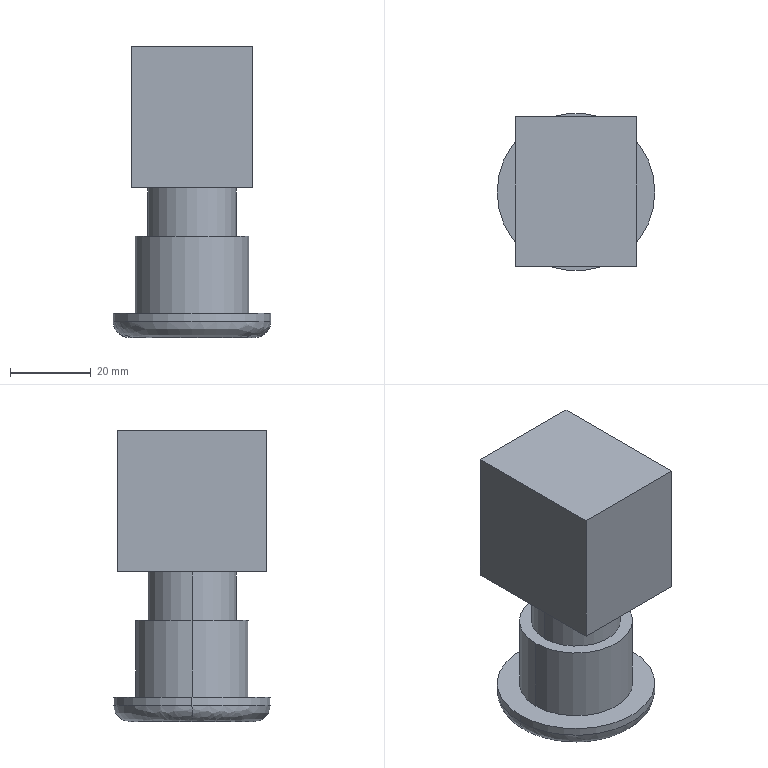Part | STEP file | Stop button AS2201 | 1 solid | 17 faces | box 39 x 39 x 72 mm | volume 61878 mm3 | plane 9 | cylinder 6 | spline 2 | commonest cylinder face diameters 22 x2 28 x2 39 x2
STEP:
#1=CARTESIAN_POINT('',(-15.5,0.,-6.));
#2=VERTEX_POINT('',#1);
#3=CARTESIAN_POINT('',(15.5,0.,-6.));
#4=VERTEX_POINT('',#3);
#5=CARTESIAN_POINT('',(-15.5,0.,-6.));
#6=CARTESIAN_POINT('',(-15.5,-31.,-6.));
#7=CARTESIAN_POINT('',(15.5,-31.,-6.));
#8=CARTESIAN_POINT('',(15.5,0.,-6.));
#9=(BOUNDED_CURVE()B_SPLINE_CURVE(3,(#5,#6,#7,#8),.UNSPECIFIED.,.F.,.T.)B_SPLINE_CURVE_WITH_KNOTS((4,4),(0.,1.),.UNSPECIFIED.)CURVE()GEOMETRIC_REPRESENTATION_ITEM()RATIONAL_B_SPLINE_CURVE((1.,0.3333,0.3333,1.))REPRESENTATION_ITEM(''));
#10=EDGE_CURVE('',#2,#4,#9,.T.);
#11=ORIENTED_EDGE('',*,*,#10,.T.);
#12=CARTESIAN_POINT('',(19.5,0.,-2.));
#13=VERTEX_POINT('',#12);
#14=CARTESIAN_POINT('',(15.5,0.,-2.));
#15=DIRECTION('',(0.,-1.,0.));
#16=DIRECTION('',(1.,0.,0.));
#17=AXIS2_PLACEMENT_3D('',#14,#15,#16);
#18=CIRCLE('',#17,4.);
#19=EDGE_CURVE('',#4,#13,#18,.T.);
#20=ORIENTED_EDGE('',*,*,#19,.T.);
#21=CARTESIAN_POINT('',(-19.5,0.,-2.));
#22=VERTEX_POINT('',#21);
#23=CARTESIAN_POINT('',(0.,0.,-2.));
#24=DIRECTION('',(0.,0.,1.));
#25=DIRECTION('',(1.,0.,0.));
#26=AXIS2_PLACEMENT_3D('',#23,#24,#25);
#27=CIRCLE('',#26,19.5);
#28=EDGE_CURVE('',#22,#13,#27,.T.);
#29=ORIENTED_EDGE('',*,*,#28,.F.);
#30=CARTESIAN_POINT('',(-15.5,0.,-2.));
#31=DIRECTION('',(0.,1.,0.));
#32=DIRECTION('',(-1.,0.,0.));
#33=AXIS2_PLACEMENT_3D('',#30,#31,#32);
#34=CIRCLE('',#33,4.);
#35=EDGE_CURVE('',#2,#22,#34,.T.);
#36=ORIENTED_EDGE('',*,*,#35,.F.);
#37=EDGE_LOOP('',(#11,#20,#29,#36));
#38=FACE_OUTER_BOUND('',#37,.T.);
#39=CARTESIAN_POINT('',(15.5,0.,-6.));
#40=CARTESIAN_POINT('',(15.5,-31.,-6.));
#41=CARTESIAN_POINT('',(-15.5,-31.,-6.));
#42=CARTESIAN_POINT('',(-15.5,0.,-6.));
#43=CARTESIAN_POINT('',(17.843,0.,-6.));
#44=CARTESIAN_POINT('',(17.843,-35.686,-6.));
#45=CARTESIAN_POINT('',(-17.843,-35.686,-6.));
#46=CARTESIAN_POINT('',(-17.843,0.,-6.));
#47=CARTESIAN_POINT('',(19.5,0.,-4.343));
#48=CARTESIAN_POINT('',(19.5,-39.,-4.343));
#49=CARTESIAN_POINT('',(-19.5,-39.,-4.343));
#50=CARTESIAN_POINT('',(-19.5,0.,-4.343));
#51=CARTESIAN_POINT('',(19.5,0.,-2.));
#52=CARTESIAN_POINT('',(19.5,-39.,-2.));
#53=CARTESIAN_POINT('',(-19.5,-39.,-2.));
#54=CARTESIAN_POINT('',(-19.5,0.,-2.));
#55=(BOUNDED_SURFACE()B_SPLINE_SURFACE(3,3,((#39,#40,#41,#42),(#43,#44,#45,#46),(#47,#48,#49,#50),(#51,#52,#53,#54)),.UNSPECIFIED.,.F.,.F.,.T.)B_SPLINE_SURFACE_WITH_KNOTS((4,4),(4,4),(0.,1.),(0.,1.),.UNSPECIFIED.)GEOMETRIC_REPRESENTATION_ITEM()RATIONAL_B_SPLINE_SURFACE(((1.,0.3333,0.3333,1.),(0.8047,0.2682,0.2682,0.8047),(0.8047,0.2682,0.2682,0.8047),(1.,0.3333,0.3333,1.)))REPRESENTATION_ITEM('')SURFACE());
#56=ADVANCED_FACE('',(#38),#55,.T.);
#57=CARTESIAN_POINT('',(11.,0.,19.));
#58=VERTEX_POINT('',#57);
#59=CARTESIAN_POINT('',(-11.,0.,19.));
#60=VERTEX_POINT('',#59);
#61=CARTESIAN_POINT('',(0.,0.,19.));
#62=DIRECTION('',(0.,0.,1.));
#63=DIRECTION('',(1.,0.,0.));
#64=AXIS2_PLACEMENT_3D('',#61,#62,#63);
#65=CIRCLE('',#64,11.);
#66=EDGE_CURVE('',#58,#60,#65,.T.);
#67=ORIENTED_EDGE('',*,*,#66,.T.);
#68=CARTESIAN_POINT('',(-11.,0.,31.));
#69=VERTEX_POINT('',#68);
#70=CARTESIAN_POINT('',(-11.,0.,19.));
#71=DIRECTION('',(0.,0.,1.));
#72=VECTOR('',#71,1000.);
#73=LINE('',#70,#72);
#74=EDGE_CURVE('',#60,#69,#73,.T.);
#75=ORIENTED_EDGE('',*,*,#74,.T.);
#76=CARTESIAN_POINT('',(11.,0.,31.));
#77=VERTEX_POINT('',#76);
#78=CARTESIAN_POINT('',(0.,0.,31.));
#79=DIRECTION('',(0.,0.,1.));
#80=DIRECTION('',(1.,0.,0.));
#81=AXIS2_PLACEMENT_3D('',#78,#79,#80);
#82=CIRCLE('',#81,11.);
#83=EDGE_CURVE('',#77,#69,#82,.T.);
#84=ORIENTED_EDGE('',*,*,#83,.F.);
#85=CARTESIAN_POINT('',(11.,0.,19.));
#86=DIRECTION('',(0.,0.,1.));
#87=VECTOR('',#86,1000.);
#88=LINE('',#85,#87);
#89=EDGE_CURVE('',#58,#77,#88,.T.);
#90=ORIENTED_EDGE('',*,*,#89,.F.);
#91=EDGE_LOOP('',(#67,#75,#84,#90));
#92=FACE_OUTER_BOUND('',#91,.T.);
#93=CARTESIAN_POINT('',(0.,0.,19.));
#94=DIRECTION('',(0.,0.,1.));
#95=DIRECTION('',(1.,0.,0.));
#96=AXIS2_PLACEMENT_3D('',#93,#94,#95);
#97=CYLINDRICAL_SURFACE('',#96,11.);
#98=ADVANCED_FACE('',(#92),#97,.T.);
#99=CARTESIAN_POINT('',(14.,0.,19.));
#100=VERTEX_POINT('',#99);
#101=CARTESIAN_POINT('',(-14.,0.,19.));
#102=VERTEX_POINT('',#101);
#103=CARTESIAN_POINT('',(0.,0.,19.));
#104=DIRECTION('',(0.,0.,1.));
#105=DIRECTION('',(-1.,0.,0.));
#106=AXIS2_PLACEMENT_3D('',#103,#104,#105);
#107=CIRCLE('',#106,14.);
#108=EDGE_CURVE('',#100,#102,#107,.T.);
#109=ORIENTED_EDGE('',*,*,#108,.F.);
#110=CARTESIAN_POINT('',(14.,0.,0.));
#111=VERTEX_POINT('',#110);
#112=CARTESIAN_POINT('',(14.,0.,31.));
#113=DIRECTION('',(0.,0.,-1.));
#114=VECTOR('',#113,1000.);
#115=LINE('',#112,#114);
#116=EDGE_CURVE('',#100,#111,#115,.T.);
#117=ORIENTED_EDGE('',*,*,#116,.T.);
#118=CARTESIAN_POINT('',(-14.,0.,0.));
#119=VERTEX_POINT('',#118);
#120=CARTESIAN_POINT('',(0.,0.,0.));
#121=DIRECTION('',(0.,0.,1.));
#122=DIRECTION('',(-1.,0.,0.));
#123=AXIS2_PLACEMENT_3D('',#120,#121,#122);
#124=CIRCLE('',#123,14.);
#125=EDGE_CURVE('',#111,#119,#124,.T.);
#126=ORIENTED_EDGE('',*,*,#125,.T.);
#127=CARTESIAN_POINT('',(-14.,0.,31.));
#128=DIRECTION('',(0.,0.,-1.));
#129=VECTOR('',#128,1000.);
#130=LINE('',#127,#129);
#131=EDGE_CURVE('',#102,#119,#130,.T.);
#132=ORIENTED_EDGE('',*,*,#131,.F.);
#133=EDGE_LOOP('',(#109,#117,#126,#132));
#134=FACE_OUTER_BOUND('',#133,.T.);
#135=CARTESIAN_POINT('',(0.,0.,31.));
#136=DIRECTION('',(0.,0.,-1.));
#137=DIRECTION('',(-1.,0.,0.));
#138=AXIS2_PLACEMENT_3D('',#135,#136,#137);
#139=CYLINDRICAL_SURFACE('',#138,14.);
#140=ADVANCED_FACE('',(#134),#139,.T.);
#141=CARTESIAN_POINT('',(0.,0.,-2.));
#142=DIRECTION('',(0.,0.,1.));
#143=DIRECTION('',(1.,0.,0.));
#144=AXIS2_PLACEMENT_3D('',#141,#142,#143);
#145=CIRCLE('',#144,19.5);
#146=EDGE_CURVE('',#13,#22,#145,.T.);
#147=ORIENTED_EDGE('',*,*,#146,.T.);
#148=CARTESIAN_POINT('',(-19.5,0.,0.));
#149=VERTEX_POINT('',#148);
#150=CARTESIAN_POINT('',(-19.5,0.,-6.));
#151=DIRECTION('',(0.,0.,1.));
#152=VECTOR('',#151,1000.);
#153=LINE('',#150,#152);
#154=EDGE_CURVE('',#22,#149,#153,.T.);
#155=ORIENTED_EDGE('',*,*,#154,.T.);
#156=CARTESIAN_POINT('',(19.5,0.,0.));
#157=VERTEX_POINT('',#156);
#158=CARTESIAN_POINT('',(0.,0.,0.));
#159=DIRECTION('',(0.,0.,-1.));
#160=DIRECTION('',(1.,0.,0.));
#161=AXIS2_PLACEMENT_3D('',#158,#159,#160);
#162=CIRCLE('',#161,19.5);
#163=EDGE_CURVE('',#149,#157,#162,.T.);
#164=ORIENTED_EDGE('',*,*,#163,.T.);
#165=CARTESIAN_POINT('',(19.5,0.,-6.));
#166=DIRECTION('',(0.,0.,1.));
#167=VECTOR('',#166,1000.);
#168=LINE('',#165,#167);
#169=EDGE_CURVE('',#13,#157,#168,.T.);
#170=ORIENTED_EDGE('',*,*,#169,.F.);
#171=EDGE_LOOP('',(#147,#155,#164,#170));
#172=FACE_OUTER_BOUND('',#171,.T.);
#173=CARTESIAN_POINT('',(0.,0.,-6.));
#174=DIRECTION('',(0.,0.,1.));
#175=DIRECTION('',(1.,0.,0.));
#176=AXIS2_PLACEMENT_3D('',#173,#174,#175);
#177=CYLINDRICAL_SURFACE('',#176,19.5);
#178=ADVANCED_FACE('',(#172),#177,.T.);
#179=CARTESIAN_POINT('',(15.,18.5,66.));
#180=VERTEX_POINT('',#179);
#181=CARTESIAN_POINT('',(15.,18.5,31.));
#182=VERTEX_POINT('',#181);
#183=CARTESIAN_POINT('',(15.,18.5,66.));
#184=DIRECTION('',(0.,0.,-1.));
#185=VECTOR('',#184,1000.);
#186=LINE('',#183,#185);
#187=EDGE_CURVE('',#180,#182,#186,.T.);
#188=ORIENTED_EDGE('',*,*,#187,.F.);
#189=CARTESIAN_POINT('',(15.,-18.5,66.));
#190=VERTEX_POINT('',#189);
#191=CARTESIAN_POINT('',(15.,-18.5,66.));
#192=DIRECTION('',(0.,1.,0.));
#193=VECTOR('',#192,1000.);
#194=LINE('',#191,#193);
#195=EDGE_CURVE('',#190,#180,#194,.T.);
#196=ORIENTED_EDGE('',*,*,#195,.F.);
#197=CARTESIAN_POINT('',(15.,-18.5,31.));
#198=VERTEX_POINT('',#197);
#199=CARTESIAN_POINT('',(15.,-18.5,66.));
#200=DIRECTION('',(0.,0.,1.));
#201=VECTOR('',#200,1000.);
#202=LINE('',#199,#201);
#203=EDGE_CURVE('',#198,#190,#202,.T.);
#204=ORIENTED_EDGE('',*,*,#203,.F.);
#205=CARTESIAN_POINT('',(15.,-18.5,31.));
#206=DIRECTION('',(0.,-1.,0.));
#207=VECTOR('',#206,1000.);
#208=LINE('',#205,#207);
#209=EDGE_CURVE('',#182,#198,#208,.T.);
#210=ORIENTED_EDGE('',*,*,#209,.F.);
#211=EDGE_LOOP('',(#188,#196,#204,#210));
#212=FACE_OUTER_BOUND('',#211,.T.);
#213=CARTESIAN_POINT('',(15.,-18.5,66.));
#214=DIRECTION('',(-1.,0.,0.));
#215=DIRECTION('',(0.,0.,1.));
#216=AXIS2_PLACEMENT_3D('',#213,#214,#215);
#217=PLANE('',#216);
#218=ADVANCED_FACE('',(#212),#217,.F.);
#219=CARTESIAN_POINT('',(-15.,-18.5,31.));
#220=VERTEX_POINT('',#219);
#221=CARTESIAN_POINT('',(-15.,18.5,31.));
#222=VERTEX_POINT('',#221);
#223=CARTESIAN_POINT('',(-15.,18.5,31.));
#224=DIRECTION('',(0.,1.,0.));
#225=VECTOR('',#224,1000.);
#226=LINE('',#223,#225);
#227=EDGE_CURVE('',#220,#222,#226,.T.);
#228=ORIENTED_EDGE('',*,*,#227,.T.);
#229=CARTESIAN_POINT('',(15.,18.5,31.));
#230=DIRECTION('',(1.,0.,0.));
#231=VECTOR('',#230,1000.);
#232=LINE('',#229,#231);
#233=EDGE_CURVE('',#222,#182,#232,.T.);
#234=ORIENTED_EDGE('',*,*,#233,.T.);
#235=ORIENTED_EDGE('',*,*,#209,.T.);
#236=CARTESIAN_POINT('',(15.,-18.5,31.));
#237=DIRECTION('',(-1.,0.,0.));
#238=VECTOR('',#237,1000.);
#239=LINE('',#236,#238);
#240=EDGE_CURVE('',#198,#220,#239,.T.);
#241=ORIENTED_EDGE('',*,*,#240,.T.);
#242=EDGE_LOOP('',(#228,#234,#235,#241));
#243=FACE_OUTER_BOUND('',#242,.T.);
#244=ORIENTED_EDGE('',*,*,#83,.T.);
#245=CARTESIAN_POINT('',(0.,0.,31.));
#246=DIRECTION('',(0.,0.,1.));
#247=DIRECTION('',(1.,0.,0.));
#248=AXIS2_PLACEMENT_3D('',#245,#246,#247);
#249=CIRCLE('',#248,11.);
#250=EDGE_CURVE('',#69,#77,#249,.T.);
#251=ORIENTED_EDGE('',*,*,#250,.T.);
#252=EDGE_LOOP('',(#244,#251));
#253=FACE_BOUND('',#252,.T.);
#254=CARTESIAN_POINT('',(15.,18.5,31.));
#255=DIRECTION('',(0.,0.,-1.));
#256=DIRECTION('',(-1.,0.,0.));
#257=AXIS2_PLACEMENT_3D('',#254,#255,#256);
#258=PLANE('',#257);
#259=ADVANCED_FACE('',(#243,#253),#258,.T.);
#260=CARTESIAN_POINT('',(-15.,18.5,66.));
#261=VERTEX_POINT('',#260);
#262=CARTESIAN_POINT('',(-15.,18.5,66.));
#263=DIRECTION('',(0.,0.,-1.));
#264=VECTOR('',#263,1000.);
#265=LINE('',#262,#264);
#266=EDGE_CURVE('',#261,#222,#265,.T.);
#267=ORIENTED_EDGE('',*,*,#266,.F.);
#268=CARTESIAN_POINT('',(-15.,18.5,66.));
#269=DIRECTION('',(-1.,0.,0.));
#270=VECTOR('',#269,1000.);
#271=LINE('',#268,#270);
#272=EDGE_CURVE('',#180,#261,#271,.T.);
#273=ORIENTED_EDGE('',*,*,#272,.F.);
#274=ORIENTED_EDGE('',*,*,#187,.T.);
#275=ORIENTED_EDGE('',*,*,#233,.F.);
#276=EDGE_LOOP('',(#267,#273,#274,#275));
#277=FACE_OUTER_BOUND('',#276,.T.);
#278=CARTESIAN_POINT('',(-15.,18.5,66.));
#279=DIRECTION('',(0.,-1.,0.));
#280=DIRECTION('',(0.,0.,-1.));
#281=AXIS2_PLACEMENT_3D('',#278,#279,#280);
#282=PLANE('',#281);
#283=ADVANCED_FACE('',(#277),#282,.F.);
#284=ORIENTED_EDGE('',*,*,#272,.T.);
#285=CARTESIAN_POINT('',(-15.,-18.5,66.));
#286=VERTEX_POINT('',#285);
#287=CARTESIAN_POINT('',(-15.,18.5,66.));
#288=DIRECTION('',(0.,1.,0.));
#289=VECTOR('',#288,1000.);
#290=LINE('',#287,#289);
#291=EDGE_CURVE('',#286,#261,#290,.T.);
#292=ORIENTED_EDGE('',*,*,#291,.F.);
#293=CARTESIAN_POINT('',(15.,-18.5,66.));
#294=DIRECTION('',(-1.,0.,0.));
#295=VECTOR('',#294,1000.);
#296=LINE('',#293,#295);
#297=EDGE_CURVE('',#190,#286,#296,.T.);
#298=ORIENTED_EDGE('',*,*,#297,.F.);
#299=ORIENTED_EDGE('',*,*,#195,.T.);
#300=EDGE_LOOP('',(#284,#292,#298,#299));
#301=FACE_OUTER_BOUND('',#300,.T.);
#302=CARTESIAN_POINT('',(15.,18.5,66.));
#303=DIRECTION('',(0.,0.,-1.));
#304=DIRECTION('',(-1.,0.,0.));
#305=AXIS2_PLACEMENT_3D('',#302,#303,#304);
#306=PLANE('',#305);
#307=ADVANCED_FACE('',(#301),#306,.F.);
#308=ORIENTED_EDGE('',*,*,#203,.T.);
#309=ORIENTED_EDGE('',*,*,#297,.T.);
#310=CARTESIAN_POINT('',(-15.,-18.5,66.));
#311=DIRECTION('',(0.,0.,1.));
#312=VECTOR('',#311,1000.);
#313=LINE('',#310,#312);
#314=EDGE_CURVE('',#220,#286,#313,.T.);
#315=ORIENTED_EDGE('',*,*,#314,.F.);
#316=ORIENTED_EDGE('',*,*,#240,.F.);
#317=EDGE_LOOP('',(#308,#309,#315,#316));
#318=FACE_OUTER_BOUND('',#317,.T.);
#319=CARTESIAN_POINT('',(-15.,-18.5,66.));
#320=DIRECTION('',(0.,1.,0.));
#321=DIRECTION('',(0.,0.,1.));
#322=AXIS2_PLACEMENT_3D('',#319,#320,#321);
#323=PLANE('',#322);
#324=ADVANCED_FACE('',(#318),#323,.F.);
#325=ORIENTED_EDGE('',*,*,#314,.T.);
#326=ORIENTED_EDGE('',*,*,#291,.T.);
#327=ORIENTED_EDGE('',*,*,#266,.T.);
#328=ORIENTED_EDGE('',*,*,#227,.F.);
#329=EDGE_LOOP('',(#325,#326,#327,#328));
#330=FACE_OUTER_BOUND('',#329,.T.);
#331=CARTESIAN_POINT('',(-15.,-18.5,66.));
#332=DIRECTION('',(1.,0.,0.));
#333=DIRECTION('',(0.,0.,-1.));
#334=AXIS2_PLACEMENT_3D('',#331,#332,#333);
#335=PLANE('',#334);
#336=ADVANCED_FACE('',(#330),#335,.F.);
#337=ORIENTED_EDGE('',*,*,#74,.F.);
#338=CARTESIAN_POINT('',(0.,0.,19.));
#339=DIRECTION('',(0.,0.,1.));
#340=DIRECTION('',(1.,0.,0.));
#341=AXIS2_PLACEMENT_3D('',#338,#339,#340);
#342=CIRCLE('',#341,11.);
#343=EDGE_CURVE('',#60,#58,#342,.T.);
#344=ORIENTED_EDGE('',*,*,#343,.T.);
#345=ORIENTED_EDGE('',*,*,#89,.T.);
#346=ORIENTED_EDGE('',*,*,#250,.F.);
#347=EDGE_LOOP('',(#337,#344,#345,#346));
#348=FACE_OUTER_BOUND('',#347,.T.);
#349=CARTESIAN_POINT('',(0.,0.,19.));
#350=DIRECTION('',(0.,0.,1.));
#351=DIRECTION('',(1.,0.,0.));
#352=AXIS2_PLACEMENT_3D('',#349,#350,#351);
#353=CYLINDRICAL_SURFACE('',#352,11.);
#354=ADVANCED_FACE('',(#348),#353,.T.);
#355=CARTESIAN_POINT('',(0.,0.,19.));
#356=DIRECTION('',(0.,0.,1.));
#357=DIRECTION('',(-1.,0.,0.));
#358=AXIS2_PLACEMENT_3D('',#355,#356,#357);
#359=CIRCLE('',#358,14.);
#360=EDGE_CURVE('',#102,#100,#359,.T.);
#361=ORIENTED_EDGE('',*,*,#360,.T.);
#362=ORIENTED_EDGE('',*,*,#108,.T.);
#363=EDGE_LOOP('',(#361,#362));
#364=FACE_OUTER_BOUND('',#363,.T.);
#365=ORIENTED_EDGE('',*,*,#66,.F.);
#366=ORIENTED_EDGE('',*,*,#343,.F.);
#367=EDGE_LOOP('',(#365,#366));
#368=FACE_BOUND('',#367,.T.);
#369=CARTESIAN_POINT('',(0.,0.,19.));
#370=DIRECTION('',(0.,0.,1.));
#371=DIRECTION('',(1.,0.,0.));
#372=AXIS2_PLACEMENT_3D('',#369,#370,#371);
#373=PLANE('',#372);
#374=ADVANCED_FACE('',(#364,#368),#373,.T.);
#375=ORIENTED_EDGE('',*,*,#116,.F.);
#376=ORIENTED_EDGE('',*,*,#360,.F.);
#377=ORIENTED_EDGE('',*,*,#131,.T.);
#378=CARTESIAN_POINT('',(0.,0.,0.));
#379=DIRECTION('',(0.,0.,1.));
#380=DIRECTION('',(-1.,0.,0.));
#381=AXIS2_PLACEMENT_3D('',#378,#379,#380);
#382=CIRCLE('',#381,14.);
#383=EDGE_CURVE('',#119,#111,#382,.T.);
#384=ORIENTED_EDGE('',*,*,#383,.T.);
#385=EDGE_LOOP('',(#375,#376,#377,#384));
#386=FACE_OUTER_BOUND('',#385,.T.);
#387=CARTESIAN_POINT('',(0.,0.,31.));
#388=DIRECTION('',(0.,0.,-1.));
#389=DIRECTION('',(-1.,0.,0.));
#390=AXIS2_PLACEMENT_3D('',#387,#388,#389);
#391=CYLINDRICAL_SURFACE('',#390,14.);
#392=ADVANCED_FACE('',(#386),#391,.T.);
#393=ORIENTED_EDGE('',*,*,#383,.F.);
#394=ORIENTED_EDGE('',*,*,#125,.F.);
#395=EDGE_LOOP('',(#393,#394));
#396=FACE_BOUND('',#395,.T.);
#397=CARTESIAN_POINT('',(0.,0.,0.));
#398=DIRECTION('',(0.,0.,-1.));
#399=DIRECTION('',(1.,0.,0.));
#400=AXIS2_PLACEMENT_3D('',#397,#398,#399);
#401=CIRCLE('',#400,19.5);
#402=EDGE_CURVE('',#157,#149,#401,.T.);
#403=ORIENTED_EDGE('',*,*,#402,.F.);
#404=ORIENTED_EDGE('',*,*,#163,.F.);
#405=EDGE_LOOP('',(#403,#404));
#406=FACE_OUTER_BOUND('',#405,.T.);
#407=CARTESIAN_POINT('',(0.,0.,0.));
#408=DIRECTION('',(0.,0.,-1.));
#409=DIRECTION('',(-1.,0.,0.));
#410=AXIS2_PLACEMENT_3D('',#407,#408,#409);
#411=PLANE('',#410);
#412=ADVANCED_FACE('',(#396,#406),#411,.F.);
#413=ORIENTED_EDGE('',*,*,#154,.F.);
#414=ORIENTED_EDGE('',*,*,#28,.T.);
#415=ORIENTED_EDGE('',*,*,#169,.T.);
#416=ORIENTED_EDGE('',*,*,#402,.T.);
#417=EDGE_LOOP('',(#413,#414,#415,#416));
#418=FACE_OUTER_BOUND('',#417,.T.);
#419=CARTESIAN_POINT('',(0.,0.,-6.));
#420=DIRECTION('',(0.,0.,1.));
#421=DIRECTION('',(1.,0.,0.));
#422=AXIS2_PLACEMENT_3D('',#419,#420,#421);
#423=CYLINDRICAL_SURFACE('',#422,19.5);
#424=ADVANCED_FACE('',(#418),#423,.T.);
#425=ORIENTED_EDGE('',*,*,#19,.F.);
#426=CARTESIAN_POINT('',(15.5,0.,-6.));
#427=CARTESIAN_POINT('',(15.5,31.,-6.));
#428=CARTESIAN_POINT('',(-15.5,31.,-6.));
#429=CARTESIAN_POINT('',(-15.5,0.,-6.));
#430=(BOUNDED_CURVE()B_SPLINE_CURVE(3,(#426,#427,#428,#429),.UNSPECIFIED.,.F.,.F.)B_SPLINE_CURVE_WITH_KNOTS((4,4),(0.,1.),.UNSPECIFIED.)CURVE()GEOMETRIC_REPRESENTATION_ITEM()RATIONAL_B_SPLINE_CURVE((1.,0.3333,0.3333,1.))REPRESENTATION_ITEM(''));
#431=EDGE_CURVE('',#4,#2,#430,.T.);
#432=ORIENTED_EDGE('',*,*,#431,.T.);
#433=ORIENTED_EDGE('',*,*,#35,.T.);
#434=ORIENTED_EDGE('',*,*,#146,.F.);
#435=EDGE_LOOP('',(#425,#432,#433,#434));
#436=FACE_OUTER_BOUND('',#435,.T.);
#437=CARTESIAN_POINT('',(-15.5,0.,-6.));
#438=CARTESIAN_POINT('',(-15.5,31.,-6.));
#439=CARTESIAN_POINT('',(15.5,31.,-6.));
#440=CARTESIAN_POINT('',(15.5,0.,-6.));
#441=CARTESIAN_POINT('',(-17.843,0.,-6.));
#442=CARTESIAN_POINT('',(-17.843,35.686,-6.));
#443=CARTESIAN_POINT('',(17.843,35.686,-6.));
#444=CARTESIAN_POINT('',(17.843,0.,-6.));
#445=CARTESIAN_POINT('',(-19.5,0.,-4.343));
#446=CARTESIAN_POINT('',(-19.5,39.,-4.343));
#447=CARTESIAN_POINT('',(19.5,39.,-4.343));
#448=CARTESIAN_POINT('',(19.5,0.,-4.343));
#449=CARTESIAN_POINT('',(-19.5,0.,-2.));
#450=CARTESIAN_POINT('',(-19.5,39.,-2.));
#451=CARTESIAN_POINT('',(19.5,39.,-2.));
#452=CARTESIAN_POINT('',(19.5,0.,-2.));
#453=(BOUNDED_SURFACE()B_SPLINE_SURFACE(3,3,((#437,#438,#439,#440),(#441,#442,#443,#444),(#445,#446,#447,#448),(#449,#450,#451,#452)),.UNSPECIFIED.,.F.,.F.,.T.)B_SPLINE_SURFACE_WITH_KNOTS((4,4),(4,4),(0.,1.),(0.,1.),.UNSPECIFIED.)GEOMETRIC_REPRESENTATION_ITEM()RATIONAL_B_SPLINE_SURFACE(((1.,0.3333,0.3333,1.),(0.8047,0.2682,0.2682,0.8047),(0.8047,0.2682,0.2682,0.8047),(1.,0.3333,0.3333,1.)))REPRESENTATION_ITEM('')SURFACE());
#454=ADVANCED_FACE('',(#436),#453,.T.);
#455=ORIENTED_EDGE('',*,*,#431,.F.);
#456=ORIENTED_EDGE('',*,*,#10,.F.);
#457=EDGE_LOOP('',(#455,#456));
#458=FACE_OUTER_BOUND('',#457,.T.);
#459=CARTESIAN_POINT('',(0.,0.,-6.));
#460=DIRECTION('',(0.,0.,-1.));
#461=DIRECTION('',(-1.,0.,0.));
#462=AXIS2_PLACEMENT_3D('',#459,#460,#461);
#463=PLANE('',#462);
#464=ADVANCED_FACE('',(#458),#463,.T.);
#465=CLOSED_SHELL('',(#56,#98,#140,#178,#218,#259,#283,#307,#324,#336,#354,#374,#392,#412,#424,#454,#464));
#466=MANIFOLD_SOLID_BREP('',#465);
#467=CARTESIAN_POINT('',(0.,0.,0.));
#468=DIRECTION('',(0.,0.,1.));
#469=DIRECTION('',(1.,0.,0.));
#470=AXIS2_PLACEMENT_3D('',#467,#468,#469);
#471=(LENGTH_UNIT()NAMED_UNIT(*)SI_UNIT(.MILLI.,.METRE.));
#472=UNCERTAINTY_MEASURE_WITH_UNIT(LENGTH_MEASURE(0.00001),#471,'','');
#473=(NAMED_UNIT(*)PLANE_ANGLE_UNIT()SI_UNIT($,.RADIAN.));
#474=(NAMED_UNIT(*)SI_UNIT($,.STERADIAN.)SOLID_ANGLE_UNIT());
#475=(GEOMETRIC_REPRESENTATION_CONTEXT(3)GLOBAL_UNCERTAINTY_ASSIGNED_CONTEXT((#472))GLOBAL_UNIT_ASSIGNED_CONTEXT((#471,#473,#474))REPRESENTATION_CONTEXT('',''));
#476=ADVANCED_BREP_SHAPE_REPRESENTATION('',(#466,#470),#475);